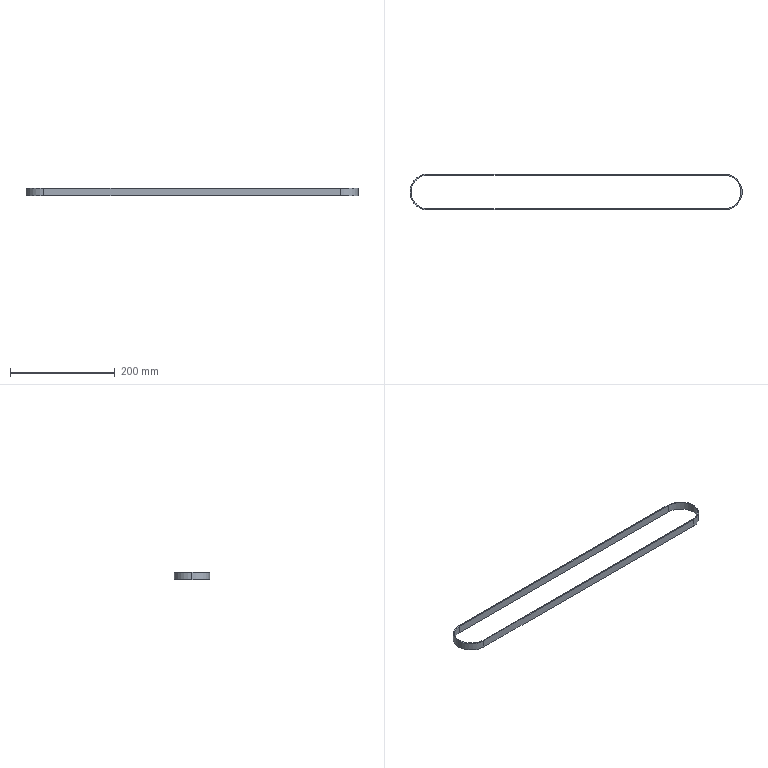Part | STEP file | 001-010-Belt 1-56 | 1 solid | 12 faces | box 635.7 x 68.7 x 15 mm | volume 40306 mm3 | cylinder 6 | plane 6 | commonest cylinder face diameters 64.7 x3 68.7 x3
STEP:
#1=CARTESIAN_POINT('',(0.,0.,0.));
#2=DIRECTION('',(0.,0.,1.));
#3=DIRECTION('',(1.,0.,0.));
#4=AXIS2_PLACEMENT_3D('',#1,#2,#3);
#5=CARTESIAN_POINT('',(-567.,32.35,7.5));
#6=VERTEX_POINT('',#5);
#7=CARTESIAN_POINT('',(-567.,32.35,-7.5));
#8=VERTEX_POINT('',#7);
#9=CARTESIAN_POINT('',(-567.,32.35,7.5));
#10=DIRECTION('',(0.,0.,-1.));
#11=VECTOR('',#10,1.);
#12=LINE('',#9,#11);
#13=CARTESIAN_POINT('',(-567.,0.,7.5));
#14=DIRECTION('',(0.,0.,-1.));
#15=DIRECTION('',(-1.,0.,0.));
#16=AXIS2_PLACEMENT_3D('',#13,#14,#15);
#17=CYLINDRICAL_SURFACE('',#16,32.35);
#18=CARTESIAN_POINT('',(1.571,0.));
#19=DIRECTION('',(0.,1.));
#20=VECTOR('',#19,1.);
#21=LINE('',#18,#20);
#22=(GEOMETRIC_REPRESENTATION_CONTEXT(2)PARAMETRIC_REPRESENTATION_CONTEXT()REPRESENTATION_CONTEXT('',''));
#23=DEFINITIONAL_REPRESENTATION('',(#21),#22);
#24=PCURVE('',#17,#23);
#25=CARTESIAN_POINT('',(-567.,32.35,7.5));
#26=DIRECTION('',(0.,-1.,0.));
#27=DIRECTION('',(1.,0.,0.));
#28=AXIS2_PLACEMENT_3D('',#25,#26,#27);
#29=PLANE('',#28);
#30=CARTESIAN_POINT('',(0.,0.));
#31=DIRECTION('',(0.,-1.));
#32=VECTOR('',#31,1.);
#33=LINE('',#30,#32);
#34=(GEOMETRIC_REPRESENTATION_CONTEXT(2)PARAMETRIC_REPRESENTATION_CONTEXT()REPRESENTATION_CONTEXT('',''));
#35=DEFINITIONAL_REPRESENTATION('',(#33),#34);
#36=PCURVE('',#29,#35);
#37=SURFACE_CURVE('',#12,(#24,#36),.PCURVE_S1.);
#38=EDGE_CURVE('',#6,#8,#37,.T.);
#39=ORIENTED_EDGE('',*,*,#38,.T.);
#40=CARTESIAN_POINT('',(-599.35,0.,-7.5));
#41=VERTEX_POINT('',#40);
#42=CARTESIAN_POINT('',(-567.,0.,-7.5));
#43=DIRECTION('',(0.,0.,1.));
#44=DIRECTION('',(-1.,0.,0.));
#45=AXIS2_PLACEMENT_3D('',#42,#43,#44);
#46=CIRCLE('',#45,32.35);
#47=CARTESIAN_POINT('',(6.283,15.));
#48=DIRECTION('',(-1.,0.));
#49=VECTOR('',#48,1.);
#50=LINE('',#47,#49);
#51=(GEOMETRIC_REPRESENTATION_CONTEXT(2)PARAMETRIC_REPRESENTATION_CONTEXT()REPRESENTATION_CONTEXT('',''));
#52=DEFINITIONAL_REPRESENTATION('',(#50),#51);
#53=PCURVE('',#17,#52);
#54=CARTESIAN_POINT('',(0.,0.,-7.5));
#55=DIRECTION('',(0.,0.,-1.));
#56=DIRECTION('',(-1.,0.,0.));
#57=AXIS2_PLACEMENT_3D('',#54,#55,#56);
#58=PLANE('',#57);
#59=CARTESIAN_POINT('',(599.35,0.));
#60=CARTESIAN_POINT('',(599.35,-56.032));
#61=CARTESIAN_POINT('',(550.825,-28.016));
#62=CARTESIAN_POINT('',(502.3,0.));
#63=CARTESIAN_POINT('',(550.825,28.016));
#64=CARTESIAN_POINT('',(599.35,56.032));
#65=CARTESIAN_POINT('',(599.35,0.));
#66=(BOUNDED_CURVE()B_SPLINE_CURVE(2,(#59,#60,#61,#62,#63,#64,#65),.UNSPECIFIED.,.T.,.F.)B_SPLINE_CURVE_WITH_KNOTS((1,2,2,2,2,1),(-2.094,0.,2.094,4.189,6.283,8.378),.UNSPECIFIED.)CURVE()GEOMETRIC_REPRESENTATION_ITEM()RATIONAL_B_SPLINE_CURVE((1.,0.5,1.,0.5,1.,0.5,1.))REPRESENTATION_ITEM(''));
#67=(GEOMETRIC_REPRESENTATION_CONTEXT(2)PARAMETRIC_REPRESENTATION_CONTEXT()REPRESENTATION_CONTEXT('',''));
#68=DEFINITIONAL_REPRESENTATION('',(#66),#67);
#69=PCURVE('',#58,#68);
#70=SURFACE_CURVE('',#46,(#53,#69),.PCURVE_S1.);
#71=EDGE_CURVE('',#8,#41,#70,.T.);
#72=ORIENTED_EDGE('',*,*,#71,.T.);
#73=CARTESIAN_POINT('',(-599.35,0.,7.5));
#74=VERTEX_POINT('',#73);
#75=CARTESIAN_POINT('',(-599.35,0.,7.5));
#76=DIRECTION('',(0.,0.,-1.));
#77=VECTOR('',#76,1.);
#78=LINE('',#75,#77);
#79=CARTESIAN_POINT('',(0.,0.));
#80=DIRECTION('',(0.,1.));
#81=VECTOR('',#80,1.);
#82=LINE('',#79,#81);
#83=(GEOMETRIC_REPRESENTATION_CONTEXT(2)PARAMETRIC_REPRESENTATION_CONTEXT()REPRESENTATION_CONTEXT('',''));
#84=DEFINITIONAL_REPRESENTATION('',(#82),#83);
#85=PCURVE('',#17,#84);
#86=CARTESIAN_POINT('',(-567.,0.,7.5));
#87=DIRECTION('',(0.,0.,-1.));
#88=DIRECTION('',(-1.,0.,0.));
#89=AXIS2_PLACEMENT_3D('',#86,#87,#88);
#90=CYLINDRICAL_SURFACE('',#89,32.35);
#91=CARTESIAN_POINT('',(6.283,0.));
#92=DIRECTION('',(0.,1.));
#93=VECTOR('',#92,1.);
#94=LINE('',#91,#93);
#95=(GEOMETRIC_REPRESENTATION_CONTEXT(2)PARAMETRIC_REPRESENTATION_CONTEXT()REPRESENTATION_CONTEXT('',''));
#96=DEFINITIONAL_REPRESENTATION('',(#94),#95);
#97=PCURVE('',#90,#96);
#98=SURFACE_CURVE('',#78,(#85,#97),.PCURVE_S1.);
#99=EDGE_CURVE('',#74,#41,#98,.T.);
#100=ORIENTED_EDGE('',*,*,#99,.F.);
#101=CARTESIAN_POINT('',(-567.,0.,7.5));
#102=DIRECTION('',(0.,0.,1.));
#103=DIRECTION('',(-1.,0.,0.));
#104=AXIS2_PLACEMENT_3D('',#101,#102,#103);
#105=CIRCLE('',#104,32.35);
#106=CARTESIAN_POINT('',(6.283,0.));
#107=DIRECTION('',(-1.,0.));
#108=VECTOR('',#107,1.);
#109=LINE('',#106,#108);
#110=(GEOMETRIC_REPRESENTATION_CONTEXT(2)PARAMETRIC_REPRESENTATION_CONTEXT()REPRESENTATION_CONTEXT('',''));
#111=DEFINITIONAL_REPRESENTATION('',(#109),#110);
#112=PCURVE('',#17,#111);
#113=CARTESIAN_POINT('',(0.,0.,7.5));
#114=DIRECTION('',(0.,0.,-1.));
#115=DIRECTION('',(-1.,0.,0.));
#116=AXIS2_PLACEMENT_3D('',#113,#114,#115);
#117=PLANE('',#116);
#118=CARTESIAN_POINT('',(599.35,0.));
#119=CARTESIAN_POINT('',(599.35,-56.032));
#120=CARTESIAN_POINT('',(550.825,-28.016));
#121=CARTESIAN_POINT('',(502.3,0.));
#122=CARTESIAN_POINT('',(550.825,28.016));
#123=CARTESIAN_POINT('',(599.35,56.032));
#124=CARTESIAN_POINT('',(599.35,0.));
#125=(BOUNDED_CURVE()B_SPLINE_CURVE(2,(#118,#119,#120,#121,#122,#123,#124),.UNSPECIFIED.,.T.,.F.)B_SPLINE_CURVE_WITH_KNOTS((1,2,2,2,2,1),(-2.094,0.,2.094,4.189,6.283,8.378),.UNSPECIFIED.)CURVE()GEOMETRIC_REPRESENTATION_ITEM()RATIONAL_B_SPLINE_CURVE((1.,0.5,1.,0.5,1.,0.5,1.))REPRESENTATION_ITEM(''));
#126=(GEOMETRIC_REPRESENTATION_CONTEXT(2)PARAMETRIC_REPRESENTATION_CONTEXT()REPRESENTATION_CONTEXT('',''));
#127=DEFINITIONAL_REPRESENTATION('',(#125),#126);
#128=PCURVE('',#117,#127);
#129=SURFACE_CURVE('',#105,(#112,#128),.PCURVE_S1.);
#130=EDGE_CURVE('',#6,#74,#129,.T.);
#131=ORIENTED_EDGE('',*,*,#130,.F.);
#132=EDGE_LOOP('',(#39,#72,#100,#131));
#133=FACE_BOUND('',#132,.F.);
#134=ADVANCED_FACE('',(#133),#17,.F.);
#135=CARTESIAN_POINT('',(-601.35,0.,7.5));
#136=VERTEX_POINT('',#135);
#137=CARTESIAN_POINT('',(-567.,-34.35,7.5));
#138=VERTEX_POINT('',#137);
#139=CARTESIAN_POINT('',(-567.,0.,7.5));
#140=DIRECTION('',(0.,0.,1.));
#141=DIRECTION('',(-1.,0.,0.));
#142=AXIS2_PLACEMENT_3D('',#139,#140,#141);
#143=CIRCLE('',#142,34.35);
#144=CARTESIAN_POINT('',(-567.,0.,7.5));
#145=DIRECTION('',(0.,0.,-1.));
#146=DIRECTION('',(-1.,0.,0.));
#147=AXIS2_PLACEMENT_3D('',#144,#145,#146);
#148=CYLINDRICAL_SURFACE('',#147,34.35);
#149=CARTESIAN_POINT('',(6.283,0.));
#150=DIRECTION('',(-1.,0.));
#151=VECTOR('',#150,1.);
#152=LINE('',#149,#151);
#153=(GEOMETRIC_REPRESENTATION_CONTEXT(2)PARAMETRIC_REPRESENTATION_CONTEXT()REPRESENTATION_CONTEXT('',''));
#154=DEFINITIONAL_REPRESENTATION('',(#152),#153);
#155=PCURVE('',#148,#154);
#156=CARTESIAN_POINT('',(601.35,0.));
#157=CARTESIAN_POINT('',(601.35,-59.496));
#158=CARTESIAN_POINT('',(549.825,-29.748));
#159=CARTESIAN_POINT('',(498.3,0.));
#160=CARTESIAN_POINT('',(549.825,29.748));
#161=CARTESIAN_POINT('',(601.35,59.496));
#162=CARTESIAN_POINT('',(601.35,0.));
#163=(BOUNDED_CURVE()B_SPLINE_CURVE(2,(#156,#157,#158,#159,#160,#161,#162),.UNSPECIFIED.,.T.,.F.)B_SPLINE_CURVE_WITH_KNOTS((1,2,2,2,2,1),(-2.094,0.,2.094,4.189,6.283,8.378),.UNSPECIFIED.)CURVE()GEOMETRIC_REPRESENTATION_ITEM()RATIONAL_B_SPLINE_CURVE((1.,0.5,1.,0.5,1.,0.5,1.))REPRESENTATION_ITEM(''));
#164=(GEOMETRIC_REPRESENTATION_CONTEXT(2)PARAMETRIC_REPRESENTATION_CONTEXT()REPRESENTATION_CONTEXT('',''));
#165=DEFINITIONAL_REPRESENTATION('',(#163),#164);
#166=PCURVE('',#117,#165);
#167=SURFACE_CURVE('',#143,(#155,#166),.PCURVE_S1.);
#168=EDGE_CURVE('',#136,#138,#167,.T.);
#169=ORIENTED_EDGE('',*,*,#168,.F.);
#170=CARTESIAN_POINT('',(-601.35,0.,-7.5));
#171=VERTEX_POINT('',#170);
#172=CARTESIAN_POINT('',(-601.35,0.,7.5));
#173=DIRECTION('',(0.,0.,-1.));
#174=VECTOR('',#173,1.);
#175=LINE('',#172,#174);
#176=CARTESIAN_POINT('',(6.283,0.));
#177=DIRECTION('',(0.,1.));
#178=VECTOR('',#177,1.);
#179=LINE('',#176,#178);
#180=(GEOMETRIC_REPRESENTATION_CONTEXT(2)PARAMETRIC_REPRESENTATION_CONTEXT()REPRESENTATION_CONTEXT('',''));
#181=DEFINITIONAL_REPRESENTATION('',(#179),#180);
#182=PCURVE('',#148,#181);
#183=CARTESIAN_POINT('',(-567.,0.,7.5));
#184=DIRECTION('',(0.,0.,-1.));
#185=DIRECTION('',(-1.,0.,0.));
#186=AXIS2_PLACEMENT_3D('',#183,#184,#185);
#187=CYLINDRICAL_SURFACE('',#186,34.35);
#188=CARTESIAN_POINT('',(0.,0.));
#189=DIRECTION('',(0.,1.));
#190=VECTOR('',#189,1.);
#191=LINE('',#188,#190);
#192=(GEOMETRIC_REPRESENTATION_CONTEXT(2)PARAMETRIC_REPRESENTATION_CONTEXT()REPRESENTATION_CONTEXT('',''));
#193=DEFINITIONAL_REPRESENTATION('',(#191),#192);
#194=PCURVE('',#187,#193);
#195=SURFACE_CURVE('',#175,(#182,#194),.PCURVE_S1.);
#196=EDGE_CURVE('',#136,#171,#195,.T.);
#197=ORIENTED_EDGE('',*,*,#196,.T.);
#198=CARTESIAN_POINT('',(-567.,-34.35,-7.5));
#199=VERTEX_POINT('',#198);
#200=CARTESIAN_POINT('',(-567.,0.,-7.5));
#201=DIRECTION('',(0.,0.,1.));
#202=DIRECTION('',(-1.,0.,0.));
#203=AXIS2_PLACEMENT_3D('',#200,#201,#202);
#204=CIRCLE('',#203,34.35);
#205=CARTESIAN_POINT('',(6.283,15.));
#206=DIRECTION('',(-1.,0.));
#207=VECTOR('',#206,1.);
#208=LINE('',#205,#207);
#209=(GEOMETRIC_REPRESENTATION_CONTEXT(2)PARAMETRIC_REPRESENTATION_CONTEXT()REPRESENTATION_CONTEXT('',''));
#210=DEFINITIONAL_REPRESENTATION('',(#208),#209);
#211=PCURVE('',#148,#210);
#212=CARTESIAN_POINT('',(601.35,0.));
#213=CARTESIAN_POINT('',(601.35,-59.496));
#214=CARTESIAN_POINT('',(549.825,-29.748));
#215=CARTESIAN_POINT('',(498.3,0.));
#216=CARTESIAN_POINT('',(549.825,29.748));
#217=CARTESIAN_POINT('',(601.35,59.496));
#218=CARTESIAN_POINT('',(601.35,0.));
#219=(BOUNDED_CURVE()B_SPLINE_CURVE(2,(#212,#213,#214,#215,#216,#217,#218),.UNSPECIFIED.,.T.,.F.)B_SPLINE_CURVE_WITH_KNOTS((1,2,2,2,2,1),(-2.094,0.,2.094,4.189,6.283,8.378),.UNSPECIFIED.)CURVE()GEOMETRIC_REPRESENTATION_ITEM()RATIONAL_B_SPLINE_CURVE((1.,0.5,1.,0.5,1.,0.5,1.))REPRESENTATION_ITEM(''));
#220=(GEOMETRIC_REPRESENTATION_CONTEXT(2)PARAMETRIC_REPRESENTATION_CONTEXT()REPRESENTATION_CONTEXT('',''));
#221=DEFINITIONAL_REPRESENTATION('',(#219),#220);
#222=PCURVE('',#58,#221);
#223=SURFACE_CURVE('',#204,(#211,#222),.PCURVE_S1.);
#224=EDGE_CURVE('',#171,#199,#223,.T.);
#225=ORIENTED_EDGE('',*,*,#224,.T.);
#226=CARTESIAN_POINT('',(-567.,-34.35,7.5));
#227=DIRECTION('',(0.,0.,-1.));
#228=VECTOR('',#227,1.);
#229=LINE('',#226,#228);
#230=CARTESIAN_POINT('',(4.712,0.));
#231=DIRECTION('',(0.,1.));
#232=VECTOR('',#231,1.);
#233=LINE('',#230,#232);
#234=(GEOMETRIC_REPRESENTATION_CONTEXT(2)PARAMETRIC_REPRESENTATION_CONTEXT()REPRESENTATION_CONTEXT('',''));
#235=DEFINITIONAL_REPRESENTATION('',(#233),#234);
#236=PCURVE('',#148,#235);
#237=CARTESIAN_POINT('',(0.,-34.35,7.5));
#238=DIRECTION('',(0.,1.,0.));
#239=DIRECTION('',(-1.,0.,0.));
#240=AXIS2_PLACEMENT_3D('',#237,#238,#239);
#241=PLANE('',#240);
#242=CARTESIAN_POINT('',(567.,0.));
#243=DIRECTION('',(0.,-1.));
#244=VECTOR('',#243,1.);
#245=LINE('',#242,#244);
#246=(GEOMETRIC_REPRESENTATION_CONTEXT(2)PARAMETRIC_REPRESENTATION_CONTEXT()REPRESENTATION_CONTEXT('',''));
#247=DEFINITIONAL_REPRESENTATION('',(#245),#246);
#248=PCURVE('',#241,#247);
#249=SURFACE_CURVE('',#229,(#236,#248),.PCURVE_S1.);
#250=EDGE_CURVE('',#138,#199,#249,.T.);
#251=ORIENTED_EDGE('',*,*,#250,.F.);
#252=EDGE_LOOP('',(#169,#197,#225,#251));
#253=FACE_BOUND('',#252,.T.);
#254=ADVANCED_FACE('',(#253),#148,.T.);
#255=CARTESIAN_POINT('',(0.,-34.35,7.5));
#256=VERTEX_POINT('',#255);
#257=CARTESIAN_POINT('',(0.,34.35,7.5));
#258=VERTEX_POINT('',#257);
#259=CARTESIAN_POINT('',(0.,0.,7.5));
#260=DIRECTION('',(0.,0.,1.));
#261=DIRECTION('',(-1.,0.,0.));
#262=AXIS2_PLACEMENT_3D('',#259,#260,#261);
#263=CIRCLE('',#262,34.35);
#264=CARTESIAN_POINT('',(34.35,0.));
#265=CARTESIAN_POINT('',(34.35,-59.496));
#266=CARTESIAN_POINT('',(-17.175,-29.748));
#267=CARTESIAN_POINT('',(-68.7,0.));
#268=CARTESIAN_POINT('',(-17.175,29.748));
#269=CARTESIAN_POINT('',(34.35,59.496));
#270=CARTESIAN_POINT('',(34.35,0.));
#271=(BOUNDED_CURVE()B_SPLINE_CURVE(2,(#264,#265,#266,#267,#268,#269,#270),.UNSPECIFIED.,.T.,.F.)B_SPLINE_CURVE_WITH_KNOTS((1,2,2,2,2,1),(-2.094,0.,2.094,4.189,6.283,8.378),.UNSPECIFIED.)CURVE()GEOMETRIC_REPRESENTATION_ITEM()RATIONAL_B_SPLINE_CURVE((1.,0.5,1.,0.5,1.,0.5,1.))REPRESENTATION_ITEM(''));
#272=(GEOMETRIC_REPRESENTATION_CONTEXT(2)PARAMETRIC_REPRESENTATION_CONTEXT()REPRESENTATION_CONTEXT('',''));
#273=DEFINITIONAL_REPRESENTATION('',(#271),#272);
#274=PCURVE('',#117,#273);
#275=CARTESIAN_POINT('',(0.,0.,7.5));
#276=DIRECTION('',(0.,0.,-1.));
#277=DIRECTION('',(-1.,0.,0.));
#278=AXIS2_PLACEMENT_3D('',#275,#276,#277);
#279=CYLINDRICAL_SURFACE('',#278,34.35);
#280=CARTESIAN_POINT('',(6.283,0.));
#281=DIRECTION('',(-1.,0.));
#282=VECTOR('',#281,1.);
#283=LINE('',#280,#282);
#284=(GEOMETRIC_REPRESENTATION_CONTEXT(2)PARAMETRIC_REPRESENTATION_CONTEXT()REPRESENTATION_CONTEXT('',''));
#285=DEFINITIONAL_REPRESENTATION('',(#283),#284);
#286=PCURVE('',#279,#285);
#287=SURFACE_CURVE('',#263,(#274,#286),.PCURVE_S1.);
#288=EDGE_CURVE('',#256,#258,#287,.T.);
#289=ORIENTED_EDGE('',*,*,#288,.T.);
#290=CARTESIAN_POINT('',(-567.,34.35,7.5));
#291=VERTEX_POINT('',#290);
#292=CARTESIAN_POINT('',(0.,34.35,7.5));
#293=DIRECTION('',(-1.,0.,0.));
#294=VECTOR('',#293,1.);
#295=LINE('',#292,#294);
#296=CARTESIAN_POINT('',(0.,34.35));
#297=DIRECTION('',(1.,0.));
#298=VECTOR('',#297,1.);
#299=LINE('',#296,#298);
#300=(GEOMETRIC_REPRESENTATION_CONTEXT(2)PARAMETRIC_REPRESENTATION_CONTEXT()REPRESENTATION_CONTEXT('',''));
#301=DEFINITIONAL_REPRESENTATION('',(#299),#300);
#302=PCURVE('',#117,#301);
#303=CARTESIAN_POINT('',(0.,34.35,7.5));
#304=DIRECTION('',(0.,-1.,0.));
#305=DIRECTION('',(1.,0.,0.));
#306=AXIS2_PLACEMENT_3D('',#303,#304,#305);
#307=PLANE('',#306);
#308=CARTESIAN_POINT('',(0.,0.));
#309=DIRECTION('',(-1.,0.));
#310=VECTOR('',#309,1.);
#311=LINE('',#308,#310);
#312=(GEOMETRIC_REPRESENTATION_CONTEXT(2)PARAMETRIC_REPRESENTATION_CONTEXT()REPRESENTATION_CONTEXT('',''));
#313=DEFINITIONAL_REPRESENTATION('',(#311),#312);
#314=PCURVE('',#307,#313);
#315=SURFACE_CURVE('',#295,(#302,#314),.PCURVE_S1.);
#316=EDGE_CURVE('',#258,#291,#315,.T.);
#317=ORIENTED_EDGE('',*,*,#316,.T.);
#318=CARTESIAN_POINT('',(-567.,0.,7.5));
#319=DIRECTION('',(0.,0.,1.));
#320=DIRECTION('',(-1.,0.,0.));
#321=AXIS2_PLACEMENT_3D('',#318,#319,#320);
#322=CIRCLE('',#321,34.35);
#323=CARTESIAN_POINT('',(601.35,0.));
#324=CARTESIAN_POINT('',(601.35,-59.496));
#325=CARTESIAN_POINT('',(549.825,-29.748));
#326=CARTESIAN_POINT('',(498.3,0.));
#327=CARTESIAN_POINT('',(549.825,29.748));
#328=CARTESIAN_POINT('',(601.35,59.496));
#329=CARTESIAN_POINT('',(601.35,0.));
#330=(BOUNDED_CURVE()B_SPLINE_CURVE(2,(#323,#324,#325,#326,#327,#328,#329),.UNSPECIFIED.,.T.,.F.)B_SPLINE_CURVE_WITH_KNOTS((1,2,2,2,2,1),(-2.094,0.,2.094,4.189,6.283,8.378),.UNSPECIFIED.)CURVE()GEOMETRIC_REPRESENTATION_ITEM()RATIONAL_B_SPLINE_CURVE((1.,0.5,1.,0.5,1.,0.5,1.))REPRESENTATION_ITEM(''));
#331=(GEOMETRIC_REPRESENTATION_CONTEXT(2)PARAMETRIC_REPRESENTATION_CONTEXT()REPRESENTATION_CONTEXT('',''));
#332=DEFINITIONAL_REPRESENTATION('',(#330),#331);
#333=PCURVE('',#117,#332);
#334=CARTESIAN_POINT('',(6.283,0.));
#335=DIRECTION('',(-1.,0.));
#336=VECTOR('',#335,1.);
#337=LINE('',#334,#336);
#338=(GEOMETRIC_REPRESENTATION_CONTEXT(2)PARAMETRIC_REPRESENTATION_CONTEXT()REPRESENTATION_CONTEXT('',''));
#339=DEFINITIONAL_REPRESENTATION('',(#337),#338);
#340=PCURVE('',#187,#339);
#341=SURFACE_CURVE('',#322,(#333,#340),.PCURVE_S1.);
#342=EDGE_CURVE('',#291,#136,#341,.T.);
#343=ORIENTED_EDGE('',*,*,#342,.T.);
#344=ORIENTED_EDGE('',*,*,#168,.T.);
#345=CARTESIAN_POINT('',(0.,-34.35,7.5));
#346=DIRECTION('',(1.,0.,0.));
#347=VECTOR('',#346,1.);
#348=LINE('',#345,#347);
#349=CARTESIAN_POINT('',(0.,-34.35));
#350=DIRECTION('',(-1.,0.));
#351=VECTOR('',#350,1.);
#352=LINE('',#349,#351);
#353=(GEOMETRIC_REPRESENTATION_CONTEXT(2)PARAMETRIC_REPRESENTATION_CONTEXT()REPRESENTATION_CONTEXT('',''));
#354=DEFINITIONAL_REPRESENTATION('',(#352),#353);
#355=PCURVE('',#117,#354);
#356=CARTESIAN_POINT('',(0.,0.));
#357=DIRECTION('',(-1.,0.));
#358=VECTOR('',#357,1.);
#359=LINE('',#356,#358);
#360=(GEOMETRIC_REPRESENTATION_CONTEXT(2)PARAMETRIC_REPRESENTATION_CONTEXT()REPRESENTATION_CONTEXT('',''));
#361=DEFINITIONAL_REPRESENTATION('',(#359),#360);
#362=PCURVE('',#241,#361);
#363=SURFACE_CURVE('',#348,(#355,#362),.PCURVE_S1.);
#364=EDGE_CURVE('',#138,#256,#363,.T.);
#365=ORIENTED_EDGE('',*,*,#364,.T.);
#366=EDGE_LOOP('',(#289,#317,#343,#344,#365));
#367=FACE_BOUND('',#366,.T.);
#368=CARTESIAN_POINT('',(0.,-32.35,7.5));
#369=VERTEX_POINT('',#368);
#370=CARTESIAN_POINT('',(0.,32.35,7.5));
#371=VERTEX_POINT('',#370);
#372=CARTESIAN_POINT('',(0.,0.,7.5));
#373=DIRECTION('',(0.,0.,1.));
#374=DIRECTION('',(-1.,0.,0.));
#375=AXIS2_PLACEMENT_3D('',#372,#373,#374);
#376=CIRCLE('',#375,32.35);
#377=CARTESIAN_POINT('',(32.35,0.));
#378=CARTESIAN_POINT('',(32.35,-56.032));
#379=CARTESIAN_POINT('',(-16.175,-28.016));
#380=CARTESIAN_POINT('',(-64.7,0.));
#381=CARTESIAN_POINT('',(-16.175,28.016));
#382=CARTESIAN_POINT('',(32.35,56.032));
#383=CARTESIAN_POINT('',(32.35,0.));
#384=(BOUNDED_CURVE()B_SPLINE_CURVE(2,(#377,#378,#379,#380,#381,#382,#383),.UNSPECIFIED.,.T.,.F.)B_SPLINE_CURVE_WITH_KNOTS((1,2,2,2,2,1),(-2.094,0.,2.094,4.189,6.283,8.378),.UNSPECIFIED.)CURVE()GEOMETRIC_REPRESENTATION_ITEM()RATIONAL_B_SPLINE_CURVE((1.,0.5,1.,0.5,1.,0.5,1.))REPRESENTATION_ITEM(''));
#385=(GEOMETRIC_REPRESENTATION_CONTEXT(2)PARAMETRIC_REPRESENTATION_CONTEXT()REPRESENTATION_CONTEXT('',''));
#386=DEFINITIONAL_REPRESENTATION('',(#384),#385);
#387=PCURVE('',#117,#386);
#388=CARTESIAN_POINT('',(0.,0.,7.5));
#389=DIRECTION('',(0.,0.,-1.));
#390=DIRECTION('',(-1.,0.,0.));
#391=AXIS2_PLACEMENT_3D('',#388,#389,#390);
#392=CYLINDRICAL_SURFACE('',#391,32.35);
#393=CARTESIAN_POINT('',(6.283,0.));
#394=DIRECTION('',(-1.,0.));
#395=VECTOR('',#394,1.);
#396=LINE('',#393,#395);
#397=(GEOMETRIC_REPRESENTATION_CONTEXT(2)PARAMETRIC_REPRESENTATION_CONTEXT()REPRESENTATION_CONTEXT('',''));
#398=DEFINITIONAL_REPRESENTATION('',(#396),#397);
#399=PCURVE('',#392,#398);
#400=SURFACE_CURVE('',#376,(#387,#399),.PCURVE_S1.);
#401=EDGE_CURVE('',#369,#371,#400,.T.);
#402=ORIENTED_EDGE('',*,*,#401,.F.);
#403=CARTESIAN_POINT('',(-567.,-32.35,7.5));
#404=VERTEX_POINT('',#403);
#405=CARTESIAN_POINT('',(0.,-32.35,7.5));
#406=DIRECTION('',(1.,0.,0.));
#407=VECTOR('',#406,1.);
#408=LINE('',#405,#407);
#409=CARTESIAN_POINT('',(0.,-32.35));
#410=DIRECTION('',(-1.,0.));
#411=VECTOR('',#410,1.);
#412=LINE('',#409,#411);
#413=(GEOMETRIC_REPRESENTATION_CONTEXT(2)PARAMETRIC_REPRESENTATION_CONTEXT()REPRESENTATION_CONTEXT('',''));
#414=DEFINITIONAL_REPRESENTATION('',(#412),#413);
#415=PCURVE('',#117,#414);
#416=CARTESIAN_POINT('',(0.,-32.35,7.5));
#417=DIRECTION('',(0.,1.,0.));
#418=DIRECTION('',(-1.,0.,0.));
#419=AXIS2_PLACEMENT_3D('',#416,#417,#418);
#420=PLANE('',#419);
#421=CARTESIAN_POINT('',(0.,0.));
#422=DIRECTION('',(-1.,0.));
#423=VECTOR('',#422,1.);
#424=LINE('',#421,#423);
#425=(GEOMETRIC_REPRESENTATION_CONTEXT(2)PARAMETRIC_REPRESENTATION_CONTEXT()REPRESENTATION_CONTEXT('',''));
#426=DEFINITIONAL_REPRESENTATION('',(#424),#425);
#427=PCURVE('',#420,#426);
#428=SURFACE_CURVE('',#408,(#415,#427),.PCURVE_S1.);
#429=EDGE_CURVE('',#404,#369,#428,.T.);
#430=ORIENTED_EDGE('',*,*,#429,.F.);
#431=CARTESIAN_POINT('',(-567.,0.,7.5));
#432=DIRECTION('',(0.,0.,1.));
#433=DIRECTION('',(-1.,0.,0.));
#434=AXIS2_PLACEMENT_3D('',#431,#432,#433);
#435=CIRCLE('',#434,32.35);
#436=CARTESIAN_POINT('',(599.35,0.));
#437=CARTESIAN_POINT('',(599.35,-56.032));
#438=CARTESIAN_POINT('',(550.825,-28.016));
#439=CARTESIAN_POINT('',(502.3,0.));
#440=CARTESIAN_POINT('',(550.825,28.016));
#441=CARTESIAN_POINT('',(599.35,56.032));
#442=CARTESIAN_POINT('',(599.35,0.));
#443=(BOUNDED_CURVE()B_SPLINE_CURVE(2,(#436,#437,#438,#439,#440,#441,#442),.UNSPECIFIED.,.T.,.F.)B_SPLINE_CURVE_WITH_KNOTS((1,2,2,2,2,1),(-2.094,0.,2.094,4.189,6.283,8.378),.UNSPECIFIED.)CURVE()GEOMETRIC_REPRESENTATION_ITEM()RATIONAL_B_SPLINE_CURVE((1.,0.5,1.,0.5,1.,0.5,1.))REPRESENTATION_ITEM(''));
#444=(GEOMETRIC_REPRESENTATION_CONTEXT(2)PARAMETRIC_REPRESENTATION_CONTEXT()REPRESENTATION_CONTEXT('',''));
#445=DEFINITIONAL_REPRESENTATION('',(#443),#444);
#446=PCURVE('',#117,#445);
#447=CARTESIAN_POINT('',(6.283,0.));
#448=DIRECTION('',(-1.,0.));
#449=VECTOR('',#448,1.);
#450=LINE('',#447,#449);
#451=(GEOMETRIC_REPRESENTATION_CONTEXT(2)PARAMETRIC_REPRESENTATION_CONTEXT()REPRESENTATION_CONTEXT('',''));
#452=DEFINITIONAL_REPRESENTATION('',(#450),#451);
#453=PCURVE('',#90,#452);
#454=SURFACE_CURVE('',#435,(#446,#453),.PCURVE_S1.);
#455=EDGE_CURVE('',#74,#404,#454,.T.);
#456=ORIENTED_EDGE('',*,*,#455,.F.);
#457=ORIENTED_EDGE('',*,*,#130,.F.);
#458=CARTESIAN_POINT('',(-567.,32.35,7.5));
#459=DIRECTION('',(-1.,0.,0.));
#460=VECTOR('',#459,1.);
#461=LINE('',#458,#460);
#462=CARTESIAN_POINT('',(567.,32.35));
#463=DIRECTION('',(1.,0.));
#464=VECTOR('',#463,1.);
#465=LINE('',#462,#464);
#466=(GEOMETRIC_REPRESENTATION_CONTEXT(2)PARAMETRIC_REPRESENTATION_CONTEXT()REPRESENTATION_CONTEXT('',''));
#467=DEFINITIONAL_REPRESENTATION('',(#465),#466);
#468=PCURVE('',#117,#467);
#469=CARTESIAN_POINT('',(0.,0.));
#470=DIRECTION('',(-1.,0.));
#471=VECTOR('',#470,1.);
#472=LINE('',#469,#471);
#473=(GEOMETRIC_REPRESENTATION_CONTEXT(2)PARAMETRIC_REPRESENTATION_CONTEXT()REPRESENTATION_CONTEXT('',''));
#474=DEFINITIONAL_REPRESENTATION('',(#472),#473);
#475=PCURVE('',#29,#474);
#476=SURFACE_CURVE('',#461,(#468,#475),.PCURVE_S1.);
#477=EDGE_CURVE('',#371,#6,#476,.T.);
#478=ORIENTED_EDGE('',*,*,#477,.F.);
#479=EDGE_LOOP('',(#402,#430,#456,#457,#478));
#480=FACE_BOUND('',#479,.T.);
#481=ADVANCED_FACE('',(#367,#480),#117,.F.);
#482=CARTESIAN_POINT('',(0.,-34.35,-7.5));
#483=VERTEX_POINT('',#482);
#484=CARTESIAN_POINT('',(0.,34.35,-7.5));
#485=VERTEX_POINT('',#484);
#486=CARTESIAN_POINT('',(0.,0.,-7.5));
#487=DIRECTION('',(0.,0.,1.));
#488=DIRECTION('',(-1.,0.,0.));
#489=AXIS2_PLACEMENT_3D('',#486,#487,#488);
#490=CIRCLE('',#489,34.35);
#491=CARTESIAN_POINT('',(34.35,0.));
#492=CARTESIAN_POINT('',(34.35,-59.496));
#493=CARTESIAN_POINT('',(-17.175,-29.748));
#494=CARTESIAN_POINT('',(-68.7,0.));
#495=CARTESIAN_POINT('',(-17.175,29.748));
#496=CARTESIAN_POINT('',(34.35,59.496));
#497=CARTESIAN_POINT('',(34.35,0.));
#498=(BOUNDED_CURVE()B_SPLINE_CURVE(2,(#491,#492,#493,#494,#495,#496,#497),.UNSPECIFIED.,.T.,.F.)B_SPLINE_CURVE_WITH_KNOTS((1,2,2,2,2,1),(-2.094,0.,2.094,4.189,6.283,8.378),.UNSPECIFIED.)CURVE()GEOMETRIC_REPRESENTATION_ITEM()RATIONAL_B_SPLINE_CURVE((1.,0.5,1.,0.5,1.,0.5,1.))REPRESENTATION_ITEM(''));
#499=(GEOMETRIC_REPRESENTATION_CONTEXT(2)PARAMETRIC_REPRESENTATION_CONTEXT()REPRESENTATION_CONTEXT('',''));
#500=DEFINITIONAL_REPRESENTATION('',(#498),#499);
#501=PCURVE('',#58,#500);
#502=CARTESIAN_POINT('',(6.283,15.));
#503=DIRECTION('',(-1.,0.));
#504=VECTOR('',#503,1.);
#505=LINE('',#502,#504);
#506=(GEOMETRIC_REPRESENTATION_CONTEXT(2)PARAMETRIC_REPRESENTATION_CONTEXT()REPRESENTATION_CONTEXT('',''));
#507=DEFINITIONAL_REPRESENTATION('',(#505),#506);
#508=PCURVE('',#279,#507);
#509=SURFACE_CURVE('',#490,(#501,#508),.PCURVE_S1.);
#510=EDGE_CURVE('',#483,#485,#509,.T.);
#511=ORIENTED_EDGE('',*,*,#510,.F.);
#512=CARTESIAN_POINT('',(0.,-34.35,-7.5));
#513=DIRECTION('',(1.,0.,0.));
#514=VECTOR('',#513,1.);
#515=LINE('',#512,#514);
#516=CARTESIAN_POINT('',(0.,-34.35));
#517=DIRECTION('',(-1.,0.));
#518=VECTOR('',#517,1.);
#519=LINE('',#516,#518);
#520=(GEOMETRIC_REPRESENTATION_CONTEXT(2)PARAMETRIC_REPRESENTATION_CONTEXT()REPRESENTATION_CONTEXT('',''));
#521=DEFINITIONAL_REPRESENTATION('',(#519),#520);
#522=PCURVE('',#58,#521);
#523=CARTESIAN_POINT('',(0.,-15.));
#524=DIRECTION('',(-1.,0.));
#525=VECTOR('',#524,1.);
#526=LINE('',#523,#525);
#527=(GEOMETRIC_REPRESENTATION_CONTEXT(2)PARAMETRIC_REPRESENTATION_CONTEXT()REPRESENTATION_CONTEXT('',''));
#528=DEFINITIONAL_REPRESENTATION('',(#526),#527);
#529=PCURVE('',#241,#528);
#530=SURFACE_CURVE('',#515,(#522,#529),.PCURVE_S1.);
#531=EDGE_CURVE('',#199,#483,#530,.T.);
#532=ORIENTED_EDGE('',*,*,#531,.F.);
#533=ORIENTED_EDGE('',*,*,#224,.F.);
#534=CARTESIAN_POINT('',(-567.,34.35,-7.5));
#535=VERTEX_POINT('',#534);
#536=CARTESIAN_POINT('',(-567.,0.,-7.5));
#537=DIRECTION('',(0.,0.,1.));
#538=DIRECTION('',(-1.,0.,0.));
#539=AXIS2_PLACEMENT_3D('',#536,#537,#538);
#540=CIRCLE('',#539,34.35);
#541=CARTESIAN_POINT('',(601.35,0.));
#542=CARTESIAN_POINT('',(601.35,-59.496));
#543=CARTESIAN_POINT('',(549.825,-29.748));
#544=CARTESIAN_POINT('',(498.3,0.));
#545=CARTESIAN_POINT('',(549.825,29.748));
#546=CARTESIAN_POINT('',(601.35,59.496));
#547=CARTESIAN_POINT('',(601.35,0.));
#548=(BOUNDED_CURVE()B_SPLINE_CURVE(2,(#541,#542,#543,#544,#545,#546,#547),.UNSPECIFIED.,.T.,.F.)B_SPLINE_CURVE_WITH_KNOTS((1,2,2,2,2,1),(-2.094,0.,2.094,4.189,6.283,8.378),.UNSPECIFIED.)CURVE()GEOMETRIC_REPRESENTATION_ITEM()RATIONAL_B_SPLINE_CURVE((1.,0.5,1.,0.5,1.,0.5,1.))REPRESENTATION_ITEM(''));
#549=(GEOMETRIC_REPRESENTATION_CONTEXT(2)PARAMETRIC_REPRESENTATION_CONTEXT()REPRESENTATION_CONTEXT('',''));
#550=DEFINITIONAL_REPRESENTATION('',(#548),#549);
#551=PCURVE('',#58,#550);
#552=CARTESIAN_POINT('',(6.283,15.));
#553=DIRECTION('',(-1.,0.));
#554=VECTOR('',#553,1.);
#555=LINE('',#552,#554);
#556=(GEOMETRIC_REPRESENTATION_CONTEXT(2)PARAMETRIC_REPRESENTATION_CONTEXT()REPRESENTATION_CONTEXT('',''));
#557=DEFINITIONAL_REPRESENTATION('',(#555),#556);
#558=PCURVE('',#187,#557);
#559=SURFACE_CURVE('',#540,(#551,#558),.PCURVE_S1.);
#560=EDGE_CURVE('',#535,#171,#559,.T.);
#561=ORIENTED_EDGE('',*,*,#560,.F.);
#562=CARTESIAN_POINT('',(0.,34.35,-7.5));
#563=DIRECTION('',(-1.,0.,0.));
#564=VECTOR('',#563,1.);
#565=LINE('',#562,#564);
#566=CARTESIAN_POINT('',(0.,34.35));
#567=DIRECTION('',(1.,0.));
#568=VECTOR('',#567,1.);
#569=LINE('',#566,#568);
#570=(GEOMETRIC_REPRESENTATION_CONTEXT(2)PARAMETRIC_REPRESENTATION_CONTEXT()REPRESENTATION_CONTEXT('',''));
#571=DEFINITIONAL_REPRESENTATION('',(#569),#570);
#572=PCURVE('',#58,#571);
#573=CARTESIAN_POINT('',(0.,-15.));
#574=DIRECTION('',(-1.,0.));
#575=VECTOR('',#574,1.);
#576=LINE('',#573,#575);
#577=(GEOMETRIC_REPRESENTATION_CONTEXT(2)PARAMETRIC_REPRESENTATION_CONTEXT()REPRESENTATION_CONTEXT('',''));
#578=DEFINITIONAL_REPRESENTATION('',(#576),#577);
#579=PCURVE('',#307,#578);
#580=SURFACE_CURVE('',#565,(#572,#579),.PCURVE_S1.);
#581=EDGE_CURVE('',#485,#535,#580,.T.);
#582=ORIENTED_EDGE('',*,*,#581,.F.);
#583=EDGE_LOOP('',(#511,#532,#533,#561,#582));
#584=FACE_BOUND('',#583,.T.);
#585=CARTESIAN_POINT('',(-567.,-32.35,-7.5));
#586=VERTEX_POINT('',#585);
#587=CARTESIAN_POINT('',(0.,-32.35,-7.5));
#588=VERTEX_POINT('',#587);
#589=CARTESIAN_POINT('',(0.,-32.35,-7.5));
#590=DIRECTION('',(1.,0.,0.));
#591=VECTOR('',#590,1.);
#592=LINE('',#589,#591);
#593=CARTESIAN_POINT('',(0.,-32.35));
#594=DIRECTION('',(-1.,0.));
#595=VECTOR('',#594,1.);
#596=LINE('',#593,#595);
#597=(GEOMETRIC_REPRESENTATION_CONTEXT(2)PARAMETRIC_REPRESENTATION_CONTEXT()REPRESENTATION_CONTEXT('',''));
#598=DEFINITIONAL_REPRESENTATION('',(#596),#597);
#599=PCURVE('',#58,#598);
#600=CARTESIAN_POINT('',(0.,-15.));
#601=DIRECTION('',(-1.,0.));
#602=VECTOR('',#601,1.);
#603=LINE('',#600,#602);
#604=(GEOMETRIC_REPRESENTATION_CONTEXT(2)PARAMETRIC_REPRESENTATION_CONTEXT()REPRESENTATION_CONTEXT('',''));
#605=DEFINITIONAL_REPRESENTATION('',(#603),#604);
#606=PCURVE('',#420,#605);
#607=SURFACE_CURVE('',#592,(#599,#606),.PCURVE_S1.);
#608=EDGE_CURVE('',#586,#588,#607,.T.);
#609=ORIENTED_EDGE('',*,*,#608,.T.);
#610=CARTESIAN_POINT('',(0.,32.35,-7.5));
#611=VERTEX_POINT('',#610);
#612=CARTESIAN_POINT('',(0.,0.,-7.5));
#613=DIRECTION('',(0.,0.,1.));
#614=DIRECTION('',(-1.,0.,0.));
#615=AXIS2_PLACEMENT_3D('',#612,#613,#614);
#616=CIRCLE('',#615,32.35);
#617=CARTESIAN_POINT('',(32.35,0.));
#618=CARTESIAN_POINT('',(32.35,-56.032));
#619=CARTESIAN_POINT('',(-16.175,-28.016));
#620=CARTESIAN_POINT('',(-64.7,0.));
#621=CARTESIAN_POINT('',(-16.175,28.016));
#622=CARTESIAN_POINT('',(32.35,56.032));
#623=CARTESIAN_POINT('',(32.35,0.));
#624=(BOUNDED_CURVE()B_SPLINE_CURVE(2,(#617,#618,#619,#620,#621,#622,#623),.UNSPECIFIED.,.T.,.F.)B_SPLINE_CURVE_WITH_KNOTS((1,2,2,2,2,1),(-2.094,0.,2.094,4.189,6.283,8.378),.UNSPECIFIED.)CURVE()GEOMETRIC_REPRESENTATION_ITEM()RATIONAL_B_SPLINE_CURVE((1.,0.5,1.,0.5,1.,0.5,1.))REPRESENTATION_ITEM(''));
#625=(GEOMETRIC_REPRESENTATION_CONTEXT(2)PARAMETRIC_REPRESENTATION_CONTEXT()REPRESENTATION_CONTEXT('',''));
#626=DEFINITIONAL_REPRESENTATION('',(#624),#625);
#627=PCURVE('',#58,#626);
#628=CARTESIAN_POINT('',(6.283,15.));
#629=DIRECTION('',(-1.,0.));
#630=VECTOR('',#629,1.);
#631=LINE('',#628,#630);
#632=(GEOMETRIC_REPRESENTATION_CONTEXT(2)PARAMETRIC_REPRESENTATION_CONTEXT()REPRESENTATION_CONTEXT('',''));
#633=DEFINITIONAL_REPRESENTATION('',(#631),#632);
#634=PCURVE('',#392,#633);
#635=SURFACE_CURVE('',#616,(#627,#634),.PCURVE_S1.);
#636=EDGE_CURVE('',#588,#611,#635,.T.);
#637=ORIENTED_EDGE('',*,*,#636,.T.);
#638=CARTESIAN_POINT('',(-567.,32.35,-7.5));
#639=DIRECTION('',(-1.,0.,0.));
#640=VECTOR('',#639,1.);
#641=LINE('',#638,#640);
#642=CARTESIAN_POINT('',(567.,32.35));
#643=DIRECTION('',(1.,0.));
#644=VECTOR('',#643,1.);
#645=LINE('',#642,#644);
#646=(GEOMETRIC_REPRESENTATION_CONTEXT(2)PARAMETRIC_REPRESENTATION_CONTEXT()REPRESENTATION_CONTEXT('',''));
#647=DEFINITIONAL_REPRESENTATION('',(#645),#646);
#648=PCURVE('',#58,#647);
#649=CARTESIAN_POINT('',(0.,-15.));
#650=DIRECTION('',(-1.,0.));
#651=VECTOR('',#650,1.);
#652=LINE('',#649,#651);
#653=(GEOMETRIC_REPRESENTATION_CONTEXT(2)PARAMETRIC_REPRESENTATION_CONTEXT()REPRESENTATION_CONTEXT('',''));
#654=DEFINITIONAL_REPRESENTATION('',(#652),#653);
#655=PCURVE('',#29,#654);
#656=SURFACE_CURVE('',#641,(#648,#655),.PCURVE_S1.);
#657=EDGE_CURVE('',#611,#8,#656,.T.);
#658=ORIENTED_EDGE('',*,*,#657,.T.);
#659=ORIENTED_EDGE('',*,*,#71,.T.);
#660=CARTESIAN_POINT('',(-567.,0.,-7.5));
#661=DIRECTION('',(0.,0.,1.));
#662=DIRECTION('',(-1.,0.,0.));
#663=AXIS2_PLACEMENT_3D('',#660,#661,#662);
#664=CIRCLE('',#663,32.35);
#665=CARTESIAN_POINT('',(599.35,0.));
#666=CARTESIAN_POINT('',(599.35,-56.032));
#667=CARTESIAN_POINT('',(550.825,-28.016));
#668=CARTESIAN_POINT('',(502.3,0.));
#669=CARTESIAN_POINT('',(550.825,28.016));
#670=CARTESIAN_POINT('',(599.35,56.032));
#671=CARTESIAN_POINT('',(599.35,0.));
#672=(BOUNDED_CURVE()B_SPLINE_CURVE(2,(#665,#666,#667,#668,#669,#670,#671),.UNSPECIFIED.,.T.,.F.)B_SPLINE_CURVE_WITH_KNOTS((1,2,2,2,2,1),(-2.094,0.,2.094,4.189,6.283,8.378),.UNSPECIFIED.)CURVE()GEOMETRIC_REPRESENTATION_ITEM()RATIONAL_B_SPLINE_CURVE((1.,0.5,1.,0.5,1.,0.5,1.))REPRESENTATION_ITEM(''));
#673=(GEOMETRIC_REPRESENTATION_CONTEXT(2)PARAMETRIC_REPRESENTATION_CONTEXT()REPRESENTATION_CONTEXT('',''));
#674=DEFINITIONAL_REPRESENTATION('',(#672),#673);
#675=PCURVE('',#58,#674);
#676=CARTESIAN_POINT('',(6.283,15.));
#677=DIRECTION('',(-1.,0.));
#678=VECTOR('',#677,1.);
#679=LINE('',#676,#678);
#680=(GEOMETRIC_REPRESENTATION_CONTEXT(2)PARAMETRIC_REPRESENTATION_CONTEXT()REPRESENTATION_CONTEXT('',''));
#681=DEFINITIONAL_REPRESENTATION('',(#679),#680);
#682=PCURVE('',#90,#681);
#683=SURFACE_CURVE('',#664,(#675,#682),.PCURVE_S1.);
#684=EDGE_CURVE('',#41,#586,#683,.T.);
#685=ORIENTED_EDGE('',*,*,#684,.T.);
#686=EDGE_LOOP('',(#609,#637,#658,#659,#685));
#687=FACE_BOUND('',#686,.T.);
#688=ADVANCED_FACE('',(#584,#687),#58,.T.);
#689=ORIENTED_EDGE('',*,*,#510,.T.);
#690=CARTESIAN_POINT('',(0.,34.35,7.5));
#691=DIRECTION('',(0.,0.,-1.));
#692=VECTOR('',#691,1.);
#693=LINE('',#690,#692);
#694=CARTESIAN_POINT('',(1.571,0.));
#695=DIRECTION('',(0.,1.));
#696=VECTOR('',#695,1.);
#697=LINE('',#694,#696);
#698=(GEOMETRIC_REPRESENTATION_CONTEXT(2)PARAMETRIC_REPRESENTATION_CONTEXT()REPRESENTATION_CONTEXT('',''));
#699=DEFINITIONAL_REPRESENTATION('',(#697),#698);
#700=PCURVE('',#279,#699);
#701=CARTESIAN_POINT('',(0.,0.));
#702=DIRECTION('',(0.,-1.));
#703=VECTOR('',#702,1.);
#704=LINE('',#701,#703);
#705=(GEOMETRIC_REPRESENTATION_CONTEXT(2)PARAMETRIC_REPRESENTATION_CONTEXT()REPRESENTATION_CONTEXT('',''));
#706=DEFINITIONAL_REPRESENTATION('',(#704),#705);
#707=PCURVE('',#307,#706);
#708=SURFACE_CURVE('',#693,(#700,#707),.PCURVE_S1.);
#709=EDGE_CURVE('',#258,#485,#708,.T.);
#710=ORIENTED_EDGE('',*,*,#709,.F.);
#711=ORIENTED_EDGE('',*,*,#288,.F.);
#712=CARTESIAN_POINT('',(0.,-34.35,7.5));
#713=DIRECTION('',(0.,0.,-1.));
#714=VECTOR('',#713,1.);
#715=LINE('',#712,#714);
#716=CARTESIAN_POINT('',(4.712,0.));
#717=DIRECTION('',(0.,1.));
#718=VECTOR('',#717,1.);
#719=LINE('',#716,#718);
#720=(GEOMETRIC_REPRESENTATION_CONTEXT(2)PARAMETRIC_REPRESENTATION_CONTEXT()REPRESENTATION_CONTEXT('',''));
#721=DEFINITIONAL_REPRESENTATION('',(#719),#720);
#722=PCURVE('',#279,#721);
#723=CARTESIAN_POINT('',(0.,0.));
#724=DIRECTION('',(0.,-1.));
#725=VECTOR('',#724,1.);
#726=LINE('',#723,#725);
#727=(GEOMETRIC_REPRESENTATION_CONTEXT(2)PARAMETRIC_REPRESENTATION_CONTEXT()REPRESENTATION_CONTEXT('',''));
#728=DEFINITIONAL_REPRESENTATION('',(#726),#727);
#729=PCURVE('',#241,#728);
#730=SURFACE_CURVE('',#715,(#722,#729),.PCURVE_S1.);
#731=EDGE_CURVE('',#256,#483,#730,.T.);
#732=ORIENTED_EDGE('',*,*,#731,.T.);
#733=EDGE_LOOP('',(#689,#710,#711,#732));
#734=FACE_BOUND('',#733,.T.);
#735=ADVANCED_FACE('',(#734),#279,.T.);
#736=ORIENTED_EDGE('',*,*,#581,.T.);
#737=CARTESIAN_POINT('',(-567.,34.35,7.5));
#738=DIRECTION('',(0.,0.,-1.));
#739=VECTOR('',#738,1.);
#740=LINE('',#737,#739);
#741=CARTESIAN_POINT('',(-567.,0.));
#742=DIRECTION('',(0.,-1.));
#743=VECTOR('',#742,1.);
#744=LINE('',#741,#743);
#745=(GEOMETRIC_REPRESENTATION_CONTEXT(2)PARAMETRIC_REPRESENTATION_CONTEXT()REPRESENTATION_CONTEXT('',''));
#746=DEFINITIONAL_REPRESENTATION('',(#744),#745);
#747=PCURVE('',#307,#746);
#748=CARTESIAN_POINT('',(1.571,0.));
#749=DIRECTION('',(0.,1.));
#750=VECTOR('',#749,1.);
#751=LINE('',#748,#750);
#752=(GEOMETRIC_REPRESENTATION_CONTEXT(2)PARAMETRIC_REPRESENTATION_CONTEXT()REPRESENTATION_CONTEXT('',''));
#753=DEFINITIONAL_REPRESENTATION('',(#751),#752);
#754=PCURVE('',#187,#753);
#755=SURFACE_CURVE('',#740,(#747,#754),.PCURVE_S1.);
#756=EDGE_CURVE('',#291,#535,#755,.T.);
#757=ORIENTED_EDGE('',*,*,#756,.F.);
#758=ORIENTED_EDGE('',*,*,#316,.F.);
#759=ORIENTED_EDGE('',*,*,#709,.T.);
#760=EDGE_LOOP('',(#736,#757,#758,#759));
#761=FACE_BOUND('',#760,.T.);
#762=ADVANCED_FACE('',(#761),#307,.F.);
#763=ORIENTED_EDGE('',*,*,#196,.F.);
#764=ORIENTED_EDGE('',*,*,#342,.F.);
#765=ORIENTED_EDGE('',*,*,#756,.T.);
#766=ORIENTED_EDGE('',*,*,#560,.T.);
#767=EDGE_LOOP('',(#763,#764,#765,#766));
#768=FACE_BOUND('',#767,.T.);
#769=ADVANCED_FACE('',(#768),#187,.T.);
#770=ORIENTED_EDGE('',*,*,#531,.T.);
#771=ORIENTED_EDGE('',*,*,#731,.F.);
#772=ORIENTED_EDGE('',*,*,#364,.F.);
#773=ORIENTED_EDGE('',*,*,#250,.T.);
#774=EDGE_LOOP('',(#770,#771,#772,#773));
#775=FACE_BOUND('',#774,.T.);
#776=ADVANCED_FACE('',(#775),#241,.F.);
#777=CARTESIAN_POINT('',(0.,32.35,7.5));
#778=DIRECTION('',(0.,0.,-1.));
#779=VECTOR('',#778,1.);
#780=LINE('',#777,#779);
#781=CARTESIAN_POINT('',(1.571,0.));
#782=DIRECTION('',(0.,1.));
#783=VECTOR('',#782,1.);
#784=LINE('',#781,#783);
#785=(GEOMETRIC_REPRESENTATION_CONTEXT(2)PARAMETRIC_REPRESENTATION_CONTEXT()REPRESENTATION_CONTEXT('',''));
#786=DEFINITIONAL_REPRESENTATION('',(#784),#785);
#787=PCURVE('',#392,#786);
#788=CARTESIAN_POINT('',(567.,0.));
#789=DIRECTION('',(0.,-1.));
#790=VECTOR('',#789,1.);
#791=LINE('',#788,#790);
#792=(GEOMETRIC_REPRESENTATION_CONTEXT(2)PARAMETRIC_REPRESENTATION_CONTEXT()REPRESENTATION_CONTEXT('',''));
#793=DEFINITIONAL_REPRESENTATION('',(#791),#792);
#794=PCURVE('',#29,#793);
#795=SURFACE_CURVE('',#780,(#787,#794),.PCURVE_S1.);
#796=EDGE_CURVE('',#371,#611,#795,.T.);
#797=ORIENTED_EDGE('',*,*,#796,.F.);
#798=ORIENTED_EDGE('',*,*,#401,.F.);
#799=CARTESIAN_POINT('',(0.,-32.35,7.5));
#800=DIRECTION('',(0.,0.,-1.));
#801=VECTOR('',#800,1.);
#802=LINE('',#799,#801);
#803=CARTESIAN_POINT('',(4.712,0.));
#804=DIRECTION('',(0.,1.));
#805=VECTOR('',#804,1.);
#806=LINE('',#803,#805);
#807=(GEOMETRIC_REPRESENTATION_CONTEXT(2)PARAMETRIC_REPRESENTATION_CONTEXT()REPRESENTATION_CONTEXT('',''));
#808=DEFINITIONAL_REPRESENTATION('',(#806),#807);
#809=PCURVE('',#392,#808);
#810=CARTESIAN_POINT('',(0.,0.));
#811=DIRECTION('',(0.,-1.));
#812=VECTOR('',#811,1.);
#813=LINE('',#810,#812);
#814=(GEOMETRIC_REPRESENTATION_CONTEXT(2)PARAMETRIC_REPRESENTATION_CONTEXT()REPRESENTATION_CONTEXT('',''));
#815=DEFINITIONAL_REPRESENTATION('',(#813),#814);
#816=PCURVE('',#420,#815);
#817=SURFACE_CURVE('',#802,(#809,#816),.PCURVE_S1.);
#818=EDGE_CURVE('',#369,#588,#817,.T.);
#819=ORIENTED_EDGE('',*,*,#818,.T.);
#820=ORIENTED_EDGE('',*,*,#636,.T.);
#821=EDGE_LOOP('',(#797,#798,#819,#820));
#822=FACE_BOUND('',#821,.F.);
#823=ADVANCED_FACE('',(#822),#392,.F.);
#824=ORIENTED_EDGE('',*,*,#657,.F.);
#825=ORIENTED_EDGE('',*,*,#796,.F.);
#826=ORIENTED_EDGE('',*,*,#477,.T.);
#827=ORIENTED_EDGE('',*,*,#38,.T.);
#828=EDGE_LOOP('',(#824,#825,#826,#827));
#829=FACE_BOUND('',#828,.T.);
#830=ADVANCED_FACE('',(#829),#29,.T.);
#831=ORIENTED_EDGE('',*,*,#684,.T.);
#832=CARTESIAN_POINT('',(-567.,-32.35,7.5));
#833=DIRECTION('',(0.,0.,-1.));
#834=VECTOR('',#833,1.);
#835=LINE('',#832,#834);
#836=CARTESIAN_POINT('',(4.712,0.));
#837=DIRECTION('',(0.,1.));
#838=VECTOR('',#837,1.);
#839=LINE('',#836,#838);
#840=(GEOMETRIC_REPRESENTATION_CONTEXT(2)PARAMETRIC_REPRESENTATION_CONTEXT()REPRESENTATION_CONTEXT('',''));
#841=DEFINITIONAL_REPRESENTATION('',(#839),#840);
#842=PCURVE('',#90,#841);
#843=CARTESIAN_POINT('',(567.,0.));
#844=DIRECTION('',(0.,-1.));
#845=VECTOR('',#844,1.);
#846=LINE('',#843,#845);
#847=(GEOMETRIC_REPRESENTATION_CONTEXT(2)PARAMETRIC_REPRESENTATION_CONTEXT()REPRESENTATION_CONTEXT('',''));
#848=DEFINITIONAL_REPRESENTATION('',(#846),#847);
#849=PCURVE('',#420,#848);
#850=SURFACE_CURVE('',#835,(#842,#849),.PCURVE_S1.);
#851=EDGE_CURVE('',#404,#586,#850,.T.);
#852=ORIENTED_EDGE('',*,*,#851,.F.);
#853=ORIENTED_EDGE('',*,*,#455,.F.);
#854=ORIENTED_EDGE('',*,*,#99,.T.);
#855=EDGE_LOOP('',(#831,#852,#853,#854));
#856=FACE_BOUND('',#855,.F.);
#857=ADVANCED_FACE('',(#856),#90,.F.);
#858=ORIENTED_EDGE('',*,*,#608,.F.);
#859=ORIENTED_EDGE('',*,*,#851,.F.);
#860=ORIENTED_EDGE('',*,*,#429,.T.);
#861=ORIENTED_EDGE('',*,*,#818,.T.);
#862=EDGE_LOOP('',(#858,#859,#860,#861));
#863=FACE_BOUND('',#862,.T.);
#864=ADVANCED_FACE('',(#863),#420,.T.);
#865=CLOSED_SHELL('',(#134,#254,#481,#688,#735,#762,#769,#776,#823,#830,#857,#864));
#866=MANIFOLD_SOLID_BREP('',#865);
#867=(LENGTH_UNIT()NAMED_UNIT(*)SI_UNIT(.MILLI.,.METRE.));
#868=UNCERTAINTY_MEASURE_WITH_UNIT(LENGTH_MEASURE(0.0000001),#867,'','');
#869=(NAMED_UNIT(*)PLANE_ANGLE_UNIT()SI_UNIT($,.RADIAN.));
#870=(NAMED_UNIT(*)SI_UNIT($,.STERADIAN.)SOLID_ANGLE_UNIT());
#871=(GEOMETRIC_REPRESENTATION_CONTEXT(3)GLOBAL_UNCERTAINTY_ASSIGNED_CONTEXT((#868))GLOBAL_UNIT_ASSIGNED_CONTEXT((#867,#869,#870))REPRESENTATION_CONTEXT('',''));
#872=ADVANCED_BREP_SHAPE_REPRESENTATION('',(#4,#866),#871);